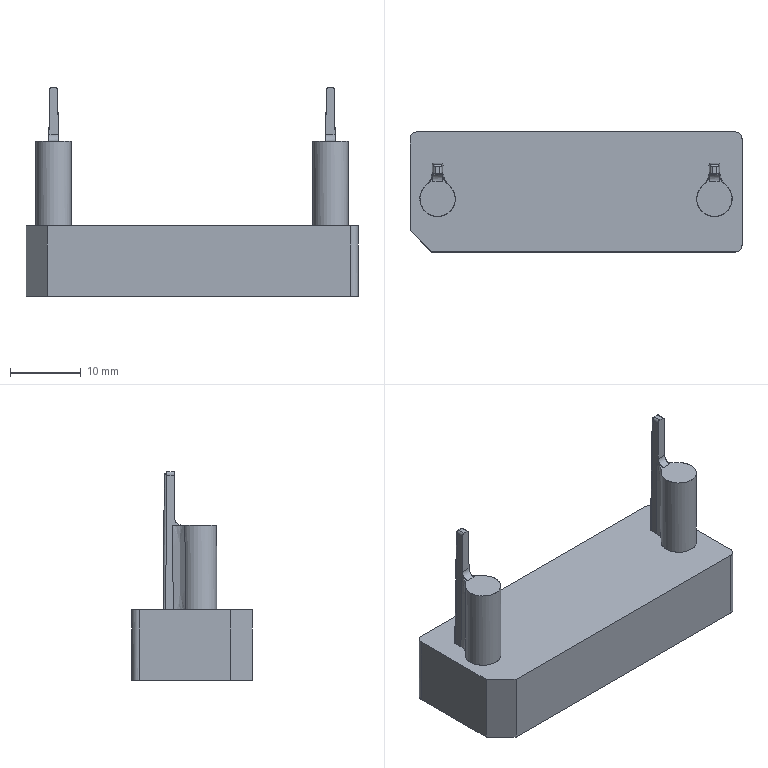NC program | PowerMill | posted with a generic post | part box 47 x 17 x 29.578 mm
Lines 11328 to 12336 of 293638:
N11425 M6
N11426 S18000 M03
N11427 G00 G90 X0.0 Y0.0
N11428 G43 Z10.798 H14
N11429
N11430 G05 P10000 R8
N11431 X21.1256 Y0.1265
N11432 Z0.908
N11433 G01 Z-0.292 F1200.0
N11434 X21.1142 Y0.1757 F2000.0
N11435 X21.0989 Y0.2239
N11436 X21.0799 Y0.2707
N11437 X21.0572 Y0.3158
N11438 X21.031 Y0.3591
N11439 X21.0015 Y0.4001
N11440 X20.9688 Y0.4387
N11441 X20.9333 Y0.4746
N11442 X20.895 Y0.5075
N11443 X20.8542 Y0.5374
N11444 X20.8112 Y0.5639
N11445 X20.7662 Y0.5869
N11446 X20.7196 Y0.6064
N11447 X20.6716 Y0.622
N11448 X20.6224 Y0.6339
N11449 X20.5725 Y0.6418
N11450 X20.5221 Y0.6458
N11451 X20.4716
N11452 X20.4212 Y0.6418
N11453 X20.3768 Y0.6349
N11454 X20.2929 Y0.6188
N11455 X20.2213 Y0.6083
N11456 X20.1571 Y0.6022
N11457 X20.094 Y0.599
N11458 X19.9708 Y0.5959
N11459 X19.8095 Y0.595
N11460 X19.4967 Y0.5949
N11461 X19.2215 Y0.5945
N11462 X19.1327 Y0.5963
N11463 X19.0442 Y0.602
N11464 X18.9562 Y0.6118
N11465 X18.8689 Y0.6254
N11466 X18.7825 Y0.643
N11467 X18.6971 Y0.6644
N11468 X18.6131 Y0.6896
N11469 X18.5304 Y0.7186
N11470 X18.4493 Y0.7512
N11471 X18.3699 Y0.7874
N11472 X18.2923 Y0.8272
N11473 X18.2163 Y0.8706
N11474 X18.1424 Y0.9174
N11475 X18.0707 Y0.9675
N11476 X18.0013 Y1.0209
N11477 X17.9345 Y1.0773
N11478 X17.8702 Y1.1367
N11479 X17.8087 Y1.1991
N11480 X17.75 Y1.2642
N11481 X17.6944 Y1.332
N11482 X17.6418 Y1.4022
N11483 X17.5925 Y1.4748
N11484 X17.5465 Y1.5496
N11485 X17.5041 Y1.6263
N11486 X17.4651 Y1.7049
N11487 X17.4298 Y1.7851
N11488 X17.3982 Y1.8667
N11489 X17.3704 Y1.9497
N11490 X17.3464 Y2.0338
N11491 X17.3262 Y2.119
N11492 X17.3098 Y2.2049
N11493 X17.2986 Y2.2821
N11494 X17.2908 Y2.3622
N11495 X17.2858 Y2.4512
N11496 X17.2838 Y2.5544
N11497 X17.2839 Y2.6866
N11498 X17.2846 Y3.3577
N11499 X17.2842 Y3.5211
N11500 X17.2858 Y3.6205
N11501 X17.2909 Y3.7136
N11502 X17.2994 Y3.8014
N11503 X17.3111 Y3.8849
N11504 X17.3262 Y3.9645
N11505 X17.3447 Y4.0428
N11506 X17.3689 Y4.1287
N11507 X17.3967 Y4.2126
N11508 X17.4279 Y4.2945
N11509 X17.4626 Y4.3742
N11510 X17.5006 Y4.4518
N11511 X17.5429 Y4.5289
N11512 X17.5885 Y4.604
N11513 X17.6376 Y4.6769
N11514 X17.6899 Y4.7476
N11515 X17.7454 Y4.8158
N11516 X17.8039 Y4.8815
N11517 X17.8654 Y4.9444
N11518 X17.9297 Y5.0045
N11519 X17.9951 Y5.0604
N11520 X18.063 Y5.1131
N11521 X18.1336 Y5.1629
N11522 X18.207 Y5.2099
N11523 X18.2831 Y5.2539
N11524 X18.3617 Y5.2947
N11525 X18.4429 Y5.3324
N11526 X18.5263 Y5.3668
N11527 X18.612 Y5.3977
N11528 X18.6997 Y5.4252
N11529 X18.7893 Y5.4491
N11530 X18.8806 Y5.4694
N11531 X18.9653 Y5.4846
N11532 X19.0519 Y5.4965
N11533 X19.1389 Y5.5046
N11534 X19.2326 Y5.5095
N11535 X19.325 Y5.5111
N11536 X19.4179 Y5.511
N11537 X19.9141 Y5.5102
N11538 X20.0031 Y5.508
N11539 X20.0929 Y5.5017
N11540 X20.1833 Y5.4914
N11541 X20.2739 Y5.4771
N11542 X20.3646 Y5.4587
N11543 X20.4551 Y5.4363
N11544 X20.5451 Y5.4099
N11545 X20.6343 Y5.3797
N11546 X20.7165 Y5.3478
N11547 X20.7971 Y5.3124
N11548 X20.8759 Y5.2733
N11549 X20.953 Y5.2307
N11550 X21.028 Y5.1847
N11551 X21.1008 Y5.1353
N11552 X21.1712 Y5.0827
N11553 X21.2392 Y5.027
N11554 X21.3045 Y4.9682
N11555 X21.3672 Y4.9066
N11556 X21.4262 Y4.843
N11557 X21.4823 Y4.7767
N11558 X21.5355 Y4.7077
N11559 X21.5856 Y4.6362
N11560 X21.6326 Y4.5622
N11561 X21.6761 Y4.4862
N11562 X21.716 Y4.4086
N11563 X21.7524 Y4.3293
N11564 X21.7851 Y4.2485
N11565 X21.8141 Y4.1661
N11566 X21.8395 Y4.0822
N11567 X21.8611 Y3.997
N11568 X21.8789 Y3.9106
N11569 X21.8929 Y3.8229
N11570 X21.903 Y3.7342
N11571 X21.9092 Y3.6445
N11572 X21.9114 Y3.5539
N11573 X21.9107 Y3.4626
N11574 X21.9103 Y3.2264
N11575 X21.9107 Y2.87
N11576 X21.9117 Y2.5975
N11577 X21.9107 Y2.492
N11578 X21.9063 Y2.3957
N11579 X21.8987 Y2.3063
N11580 X21.8878 Y2.2225
N11581 X21.8738 Y2.1433
N11582 X21.8564 Y2.065
N11583 X21.8334 Y1.9793
N11584 X21.8067 Y1.8952
N11585 X21.7764 Y1.8129
N11586 X21.7427 Y1.7326
N11587 X21.7054 Y1.6543
N11588 X21.6649 Y1.5782
N11589 X21.621 Y1.5041
N11590 X21.5723 Y1.4298
N11591 X21.5208 Y1.3582
N11592 X21.4664 Y1.2895
N11593 X21.4092 Y1.2236
N11594 X21.3493 Y1.1607
N11595 X21.2866 Y1.1006
N11596 X21.2204 Y1.0428
N11597 X21.1517 Y0.988
N11598 X21.0806 Y0.9365
N11599 X21.0073 Y0.8882
N11600 X20.9319 Y0.8433
N11601 X20.8546 Y0.802
N11602 X20.7754 Y0.7642
N11603 X20.6948 Y0.7301
N11604 X20.6126 Y0.6997
N11605 X20.529 Y0.6731
N11606 X20.4441 Y0.6502
N11607 X20.3768 Y0.6349
N11608 X20.328 Y0.6218
N11609 X20.2804 Y0.6049
N11610 X20.2343 Y0.5842
N11611 X20.1899 Y0.56
N11612 X20.1476 Y0.5324
N11613 X20.1076 Y0.5015
N11614 X20.0701 Y0.4676
N11615 X20.0355 Y0.4308
N11616 X20.0038 Y0.3914
N11617 X19.9754 Y0.3496
N11618 X19.9504 Y0.3057
N11619 X19.9289 Y0.26
N11620 X19.9111 Y0.2128
N11621 X19.897 Y0.1642
N11622 X19.8868 Y0.1147
N11623 X19.8806 Y0.0645
N11624 X19.8784 Y0.0141
N11625 X19.8801 Y-0.0364
N11626 X19.8858 Y-0.0866
N11627 X19.8942 Y-0.1308
N11628 X21.1239 Y0.1156 Z-0.312
N11629 X21.1128 Y0.1648
N11630 X21.0978 Y0.2131
N11631 X21.079 Y0.26
N11632 X21.0566 Y0.3053
N11633 X21.0306 Y0.3487
N11634 X21.0014 Y0.3899
N11635 X20.9689 Y0.4287
N11636 X20.9336 Y0.4647
N11637 X20.8955 Y0.4979
N11638 X20.8548 Y0.528
N11639 X20.812 Y0.5547
N11640 X20.7672 Y0.578
N11641 X20.7207 Y0.5977
N11642 X20.6727 Y0.6137
N11643 X20.6236 Y0.6258
N11644 X20.5737 Y0.634
N11645 X20.5234 Y0.6383
N11646 X20.4729 Y0.6386
N11647 X20.4225 Y0.6349
N11648 X20.378 Y0.6282
N11649 X20.3278 Y0.6189
N11650 X20.2419 Y0.607
N11651 X20.156 Y0.5992
N11652 X20.07 Y0.5953
N11653 X19.984 Y0.5948
N11654 X19.2215 Y0.5947
N11655 X19.1172 Y0.5963
N11656 X19.0237 Y0.6011
N11657 X18.9378 Y0.6091
N11658 X18.8579 Y0.6201
N11659 X18.7826 Y0.6342
N11660 X18.708 Y0.6516
N11661 X18.6213 Y0.6756
N11662 X18.5367 Y0.703
N11663 X18.4543 Y0.7339
N11664 X18.3743 Y0.7681
N11665 X18.2968 Y0.8055
N11666 X18.2218 Y0.846
N11667 X18.1489 Y0.8899
N11668 X18.0745 Y0.9391
N11669 X18.003 Y0.9913
N11670 X17.9344 Y1.0462
N11671 X17.8689 Y1.1037
N11672 X17.8067 Y1.1636
N11673 X17.7475 Y1.2259
N11674 X17.6898 Y1.2927
N11675 X17.6352 Y1.3619
N11676 X17.5839 Y1.4333
N11677 X17.536 Y1.5068
N11678 X17.4916 Y1.5823
N11679 X17.4508 Y1.6595
N11680 X17.4137 Y1.7383
N11681 X17.3802 Y1.8187
N11682 X17.3501 Y1.901
N11683 X17.3244 Y1.9824
N11684 X17.303 Y2.0632
N11685 X17.2872 Y2.1358
N11686 X17.2745 Y2.2051
N11687 X17.2638 Y2.2746
N11688 X17.2558 Y2.3446
N11689 X17.2509 Y2.4148
N11690 X17.2486 Y2.4853
N11691 X17.248 Y2.5558
N11692 Y2.6263
N11693 X17.2476 Y3.1941
N11694 X17.2472 Y3.521
N11695 X17.2485 Y3.6202
N11696 X17.2529 Y3.708
N11697 X17.2606 Y3.7893
N11698 X17.2727 Y3.8762
N11699 X17.2889 Y3.9625
N11700 X17.3089 Y4.048
N11701 X17.3328 Y4.1325
N11702 X17.3606 Y4.2158
N11703 X17.392 Y4.2976
N11704 X17.4272 Y4.3779
N11705 X17.4659 Y4.4565
N11706 X17.5082 Y4.5333
N11707 X17.554 Y4.608
N11708 X17.6031 Y4.6806
N11709 X17.6555 Y4.7509
N11710 X17.711 Y4.8187
N11711 X17.7695 Y4.8839
N11712 X17.8313 Y4.9469
N11713 X17.8956 Y5.0066
N11714 X17.9621 Y5.0631
N11715 X18.0308 Y5.1162
N11716 X18.1016 Y5.1661
N11717 X18.1788 Y5.2156
N11718 X18.2581 Y5.2617
N11719 X18.3395 Y5.3044
N11720 X18.4228 Y5.3437
N11721 X18.5078 Y5.3793
N11722 X18.5885 Y5.4092
N11723 X18.6702 Y5.4362
N11724 X18.7529 Y5.4598
N11725 X18.8367 Y5.4801
N11726 X18.923 Y5.4972
N11727 X19.0121 Y5.5108
N11728 X19.1042 Y5.521
N11729 X19.1995 Y5.5276
N11730 X19.2977 Y5.5306
N11731 X19.3976 Y5.5308
N11732 X19.9141 Y5.5307
N11733 X19.9966 Y5.5288
N11734 X20.0826 Y5.5228
N11735 X20.1727 Y5.5127
N11736 X20.2605 Y5.4993
N11737 X20.3508 Y5.4819
N11738 X20.4404 Y5.4606
N11739 X20.5289 Y5.4354
N11740 X20.616 Y5.4064
N11741 X20.7017 Y5.3738
N11742 X20.7857 Y5.3377
N11743 X20.8696 Y5.2975
N11744 X20.9502 Y5.2547
N11745 X21.0277 Y5.2091
N11746 X21.1021 Y5.1607
N11747 X21.1736 Y5.1096
N11748 X21.2423 Y5.0556
N11749 X21.3083 Y4.9988
N11750 X21.3716 Y4.9392
N11751 X21.4326 Y4.8765
N11752 X21.4908 Y4.8109
N11753 X21.546 Y4.7427
N11754 X21.598 Y4.672
N11755 X21.6467 Y4.5991
N11756 X21.6921 Y4.524
N11757 X21.734 Y4.4469
N11758 X21.7724 Y4.3679
N11759 X21.8072 Y4.2873
N11760 X21.8382 Y4.2053
N11761 X21.8655 Y4.1219
N11762 X21.8881 Y4.0405
N11763 X21.9071 Y3.9572
N11764 X21.9226 Y3.8715
N11765 X21.9345 Y3.7833
N11766 X21.9428 Y3.6928
N11767 X21.9473 Y3.5998
N11768 X21.9481 Y3.5043
N11769 X21.9472 Y3.1096
N11770 X21.9471 Y2.7232
N11771 X21.9475 Y2.5975
N11772 X21.9467 Y2.4897
N11773 X21.9428 Y2.3964
N11774 X21.9359 Y2.3124
N11775 X21.9258 Y2.2339
N11776 X21.9107 Y2.1474
N11777 X21.8915 Y2.0613
N11778 X21.8685 Y1.9758
N11779 X21.8421 Y1.8929
N11780 X21.812 Y1.8113
N11781 X21.7782 Y1.7311
N11782 X21.7407 Y1.6523
N11783 X21.6995 Y1.5752
N11784 X21.6547 Y1.4999
N11785 X21.6065 Y1.4265
N11786 X21.5549 Y1.3553
N11787 X21.5003 Y1.2867
N11788 X21.4426 Y1.2207
N11789 X21.3819 Y1.1573
N11790 X21.3184 Y1.0967
N11791 X21.2522 Y1.0391
N11792 X21.1835 Y0.9846
N11793 X21.1123 Y0.9332
N11794 X21.0389 Y0.8852
N11795 X20.9635 Y0.8406
N11796 X20.8861 Y0.7996
N11797 X20.8069 Y0.762
N11798 X20.726 Y0.7281
N11799 X20.6435 Y0.6978
N11800 X20.5597 Y0.6713
N11801 X20.4746 Y0.6486
N11802 X20.4137 Y0.6348
N11803 X20.378 Y0.6282
N11804 X20.3288 Y0.6171
N11805 X20.2805 Y0.6021
N11806 X20.2336 Y0.5833
N11807 X20.1883 Y0.5609
N11808 X20.1449 Y0.5349
N11809 X20.1037 Y0.5057
N11810 X20.0649 Y0.4732
N11811 X20.0289 Y0.4379
N11812 X19.9957 Y0.3998
N11813 X19.9656 Y0.3591
N11814 X19.9389 Y0.3163
N11815 X19.9156 Y0.2715
N11816 X19.8959 Y0.225
N11817 X19.8799 Y0.177
N11818 X19.8678 Y0.1279
N11819 X19.8596 Y0.078
N11820 X19.8553 Y0.0277
N11821 X19.855 Y-0.0228
N11822 X19.8587 Y-0.0732
N11823 X19.8654 Y-0.1177
N11824 X21.1241 Y0.1097 Z-0.332
N11825 X21.113 Y0.159
N11826 X21.0981 Y0.2073
N11827 X21.0794 Y0.2542
N11828 X21.057 Y0.2996
N11829 X21.0311 Y0.343
N11830 X21.0019 Y0.3843
N11831 X20.9696 Y0.4231
N11832 X20.9342 Y0.4592
N11833 X20.8962 Y0.4924
N11834 X20.8556 Y0.5225
N11835 X20.8128 Y0.5493
N11836 X20.768 Y0.5727
N11837 X20.7215 Y0.5925
N11838 X20.6736 Y0.6085
N11839 X20.6245 Y0.6207
N11840 X20.5746 Y0.629
N11841 X20.5243 Y0.6333
N11842 X20.4738 Y0.6337
N11843 X20.4234 Y0.63
N11844 X20.3789 Y0.6234
N11845 X20.3587 Y0.6197
N11846 X20.2731 Y0.608
N11847 X20.1846 Y0.5998
N11848 X20.0932 Y0.5954
N11849 X19.9986 Y0.5945
N11850 X19.6833 Y0.5944
N11851 X19.4371 Y0.5953
N11852 X19.2513 Y0.5949
N11853 X19.1478 Y0.5944
N11854 X19.0518 Y0.5973
N11855 X18.9618 Y0.6036
N11856 X18.8767 Y0.6133
N11857 X18.796 Y0.6263
N11858 X18.7172 Y0.6428
N11859 X18.6309 Y0.6648
N11860 X18.5461 Y0.6905
N11861 X18.463 Y0.7198
N11862 X18.3817 Y0.7527
N11863 X18.3024 Y0.7891
N11864 X18.2251 Y0.8289
N11865 X18.1498 Y0.8722
N11866 X18.0758 Y0.9193
N11867 X18.0041 Y0.9697
N11868 X17.9347 Y1.0233
N11869 X17.8678 Y1.08
N11870 X17.8036 Y1.1397
N11871 X17.7421 Y1.2023
N11872 X17.6836 Y1.2677
N11873 X17.628 Y1.3356
N11874 X17.5757 Y1.4059
N11875 X17.5266 Y1.4786
N11876 X17.4809 Y1.5534
N11877 X17.4386 Y1.6302
N11878 X17.3999 Y1.7088
N11879 X17.3657 Y1.787
N11880 X17.335 Y1.8668
N11881 X17.3074 Y1.9496
N11882 X17.2829 Y2.0354
N11883 X17.2617 Y2.1243
N11884 X17.2471 Y2.2004
N11885 X17.2357 Y2.2802
N11886 X17.2275 Y2.3655
N11887 X17.2224 Y2.4575
N11888 X17.2207 Y2.5587
N11889 X17.2214 Y2.6734
N11890 X17.2211 Y2.9073
N11891 X17.2206 Y3.1868
N11892 X17.2199 Y3.521
N11893 X17.2213 Y3.6149
N11894 X17.2266 Y3.707
N11895 X17.2356 Y3.7973
N11896 X17.2484 Y3.8859
N11897 X17.265 Y3.9727
N11898 X17.2852 Y4.058
N11899 X17.3091 Y4.1416
N11900 X17.3366 Y4.2236
N11901 X17.3678 Y4.3041
N11902 X17.4028 Y4.3832
N11903 X17.4415 Y4.4613
N11904 X17.4841 Y4.5381
N11905 X17.5301 Y4.6129
N11906 X17.5795 Y4.6855
N11907 X17.6321 Y4.7558
N11908 X17.6879 Y4.8237
N11909 X17.7467 Y4.889
N11910 X17.8084 Y4.9515
N11911 X17.8729 Y5.0111
N11912 X17.94 Y5.0677
N11913 X18.0095 Y5.1214
N11914 X18.0868 Y5.1764
N11915 X18.1652 Y5.2274
N11916 X18.2446 Y5.2743
N11917 X18.3248 Y5.3172
N11918 X18.4059 Y5.3561
N11919 X18.4862 Y5.3905
N11920 X18.5671 Y5.4217
N11921 X18.6491 Y5.4498
N11922 X18.7326 Y5.4746
N11923 X18.8179 Y5.4961
N11924 X18.9052 Y5.5142
N11925 X18.9948 Y5.5287
N11926 X19.0868 Y5.5396
N11927 X19.1815 Y5.5469
N11928 X19.2788 Y5.5506
N11929 X19.3785 Y5.5511
N11930 X19.9141 Y5.5506
N11931 X20.0006 Y5.5485
N11932 X20.0881 Y5.5425
N11933 X20.1774 Y5.5325
N11934 X20.2679 Y5.5184
N11935 X20.359 Y5.5002
N11936 X20.4499 Y5.478
N11937 X20.5397 Y5.4519
N11938 X20.6277 Y5.4223
N11939 X20.7131 Y5.3894
N11940 X20.7956 Y5.3534
N11941 X20.8755 Y5.3144
N11942 X20.9588 Y5.2694
N11943 X21.0397 Y5.2211
N11944 X21.1181 Y5.1697
N11945 X21.1938 Y5.1153
N11946 X21.2667 Y5.0581
N11947 X21.3328 Y5.0015
N11948 X21.3963 Y4.9419
N11949 X21.4573 Y4.8793
N11950 X21.5155 Y4.8138
N11951 X21.5708 Y4.7456
N11952 X21.623 Y4.6748
N11953 X21.672 Y4.6016
N11954 X21.7176 Y4.5263
N11955 X21.7598 Y4.449
N11956 X21.7983 Y4.3701
N11957 X21.8331 Y4.2896
N11958 X21.8642 Y4.2078
N11959 X21.891 Y4.1264
N11960 X21.914 Y4.0441
N11961 X21.9334 Y3.9603
N11962 X21.9492 Y3.875
N11963 X21.9612 Y3.788
N11964 X21.9694 Y3.6991
N11965 X21.9739 Y3.6081
N11966 X21.9747 Y3.5211
N11967 X21.9741 Y3.2959
N11968 X21.9746 Y3.0593
N11969 X21.9737 Y2.7677
N11970 X21.9741 Y2.5975
N11971 X21.9736 Y2.5078
N11972 X21.9703 Y2.4174
N11973 X21.9634 Y2.3272
N11974 X21.9531 Y2.2405
N11975 X21.9395 Y2.1574
N11976 X21.9227 Y2.0779
N11977 X21.9029 Y2.001
N11978 X21.88 Y1.925
N11979 X21.854 Y1.85
N11980 X21.8218 Y1.7689
N11981 X21.786 Y1.6893
N11982 X21.7465 Y1.6113
N11983 X21.7034 Y1.5351
N11984 X21.6568 Y1.4608
N11985 X21.6069 Y1.3886
N11986 X21.5536 Y1.3188
N11987 X21.4972 Y1.2513
N11988 X21.4378 Y1.1865
N11989 X21.3758 Y1.1248
N11990 X21.3111 Y1.0659
N11991 X21.2436 Y1.01
N11992 X21.1737 Y0.9572
N11993 X21.1014 Y0.9076
N11994 X21.0269 Y0.8613
N11995 X20.9503 Y0.8185
N11996 X20.8719 Y0.7792
N11997 X20.7918 Y0.7435
N11998 X20.7101 Y0.7116
N11999 X20.6271 Y0.6833
N12000 X20.5429 Y0.6589
N12001 X20.4577 Y0.6384
N12002 X20.4416 Y0.635
N12003 X20.3789 Y0.6234
N12004 X20.3296 Y0.6123
N12005 X20.2814 Y0.5974
N12006 X20.2344 Y0.5787
N12007 X20.1891 Y0.5563
N12008 X20.1457 Y0.5304
N12009 X20.1044 Y0.5012
N12010 X20.0656 Y0.4689
N12011 X20.0295 Y0.4335
N12012 X19.9963 Y0.3955
N12013 X19.9662 Y0.3549
N12014 X19.9393 Y0.3121
N12015 X19.916 Y0.2673
N12016 X19.8962 Y0.2208
N12017 X19.8802 Y0.1729
N12018 X19.868 Y0.1238
N12019 X19.8597 Y0.0739
N12020 X19.8554 Y0.0236
N12021 X19.855 Y-0.0269
N12022 X19.8587 Y-0.0773
N12023 X19.8652 Y-0.1218
N12024 X21.1254 Y0.1076 Z-0.352
N12025 X21.1142 Y0.1569
N12026 X21.0992 Y0.2052
N12027 X21.0804 Y0.2521
N12028 X21.058 Y0.2974
N12029 X21.0321 Y0.3408
N12030 X21.0028 Y0.382
N12031 X20.9704 Y0.4207
N12032 X20.935 Y0.4568
N12033 X20.8969 Y0.49
N12034 X20.8563 Y0.52
N12035 X20.8135 Y0.5468
N12036 X20.7686 Y0.5701
N12037 X20.7221 Y0.5898
N12038 X20.6742 Y0.6058
N12039 X20.6251 Y0.6179
N12040 X20.5752 Y0.6261
N12041 X20.5249 Y0.6304
N12042 X20.4743 Y0.6307
N12043 X20.424 Y0.627
N12044 X20.3795 Y0.6203
N12045 X20.3695 Y0.6185
N12046 X20.3048 Y0.6084
N12047 X20.2492 Y0.6028
N12048 X20.155 Y0.5975
N12049 X20.0438 Y0.5948
N12050 X19.9141 Y0.5943
N12051 X19.3369 Y0.5942
N12052 X19.1777
N12053 X19.0658 Y0.5963
N12054 X18.9723 Y0.601
N12055 X18.8894 Y0.6085
N12056 X18.8138 Y0.6188
N12057 X18.7422 Y0.6323
N12058 X18.6522 Y0.6532
N12059 X18.5652 Y0.6775
N12060 X18.4812 Y0.7049
N12061 X18.4 Y0.7355
N12062 X18.3218 Y0.7692
N12063 X18.2455 Y0.8062
N12064 X18.1686 Y0.8479
N12065 X18.0936 Y0.8931
N12066 X18.0208 Y0.9415
N12067 X17.9503 Y0.9933
N12068 X17.8821 Y1.0482
N12069 X17.8165 Y1.1062
N12070 X17.7535 Y1.1672
N12071 X17.6934 Y1.231
N12072 X17.6362 Y1.2975
N12073 X17.582 Y1.3666
N12074 X17.5311 Y1.438
N12075 X17.4835 Y1.5117
N12076 X17.4393 Y1.5874
N12077 X17.3987 Y1.665
N12078 X17.3616 Y1.7443
N12079 X17.3282 Y1.8252
N12080 X17.2985 Y1.9075
N12081 X17.2726 Y1.991
N12082 X17.2505 Y2.0757
N12083 X17.2345 Y2.1494
N12084 X17.2214 Y2.2236
N12085 X17.2114 Y2.2983
N12086 X17.2043 Y2.3761
N12087 X17.2001 Y2.4586
N12088 X17.1985 Y2.5341
N12089 X17.1983 Y2.6096
N12090 X17.1991 Y3.101
N12091 X17.1981 Y3.5211
N12092 X17.1996 Y3.6175
N12093 X17.2047 Y3.7105
N12094 X17.2135 Y3.8003
N12095 X17.2259 Y3.8871
N12096 X17.2417 Y3.971
N12097 X17.2609 Y4.0522
N12098 X17.2837 Y4.1317
N12099 X17.3121 Y4.2166
N12100 X17.3439 Y4.2992
N12101 X17.3791 Y4.3796
N12102 X17.4175 Y4.4576
N12103 X17.4591 Y4.5331
N12104 X17.5039 Y4.6062
N12105 X17.5535 Y4.6797
N12106 X17.6063 Y4.7507
N12107 X17.6622 Y4.8192
N12108 X17.7213 Y4.8854
N12109 X17.7836 Y4.9491
N12110 X17.8491 Y5.0105
N12111 X17.921 Y5.0723
N12112 X17.9951 Y5.1309
N12113 X18.0715 Y5.186
N12114 X18.1499 Y5.2378
N12115 X18.2301 Y5.286
N12116 X18.3121 Y5.3306
N12117 X18.3956 Y5.3715
N12118 X18.4806 Y5.4087
N12119 X18.5668 Y5.4421
N12120 X18.6542 Y5.4717
N12121 X18.7402 Y5.4967
N12122 X18.8271 Y5.5182
N12123 X18.9156 Y5.536
N12124 X19.0063 Y5.5503
N12125 X19.0993 Y5.5609
N12126 X19.1948 Y5.5678
N12127 X19.2931 Y5.5711
N12128 X19.3938 Y5.5713
N12129 X19.9141 Y5.5707
N12130 X20.0009 Y5.5686
N12131 X20.0887 Y5.5625
N12132 X20.1782 Y5.5525
N12133 X20.2688 Y5.5383
N12134 X20.3599 Y5.5201
N12135 X20.4509 Y5.4978
N12136 X20.5408 Y5.4717
N12137 X20.6289 Y5.442
N12138 X20.7146 Y5.4089
N12139 X20.7974 Y5.3728
N12140 X20.8777 Y5.3335
N12141 X20.9601 Y5.2889
N12142 X21.0406 Y5.2406
N12143 X21.1192 Y5.1889
N12144 X21.1956 Y5.1339
N12145 X21.2699 Y5.0755
N12146 X21.3417 Y5.0139
N12147 X21.4087 Y4.9516
N12148 X21.4706 Y4.8888
N12149 X21.5276 Y4.8255
N12150 X21.5818 Y4.7597
N12151 X21.635 Y4.689
N12152 X21.6846 Y4.6165
N12153 X21.7307 Y4.5421
N12154 X21.7731 Y4.4662
N12155 X21.8117 Y4.3888
N12156 X21.8465 Y4.3101
N12157 X21.8776 Y4.2302
N12158 X21.903 Y4.1559
N12159 X21.9257 Y4.0807
N12160 X21.9455 Y4.0047
N12161 X21.962 Y3.928
N12162 X21.9751 Y3.8503
N12163 X21.9854 Y3.7674
N12164 X21.9923 Y3.6797
N12165 X21.9957 Y3.5939
N12166 X21.9964 Y3.5102
N12167 X21.9963 Y2.9438
N12168 X21.9962 Y2.8824
N12169 Y2.8209
N12170 X21.9961 Y2.7594
N12171 X21.9959 Y2.691
N12172 X21.9957 Y2.6295
N12173 X21.9953 Y2.5681
N12174 X21.9948 Y2.5066
N12175 X21.994 Y2.4452
N12176 X21.9925 Y2.3884
N12177 X21.9884 Y2.3317
N12178 X21.9817 Y2.2753
N12179 X21.973 Y2.2174
N12180 X21.96 Y2.1465
N12181 X21.9413 Y2.0617
N12182 X21.9241 Y1.9949
N12183 X21.9079 Y1.9404
N12184 X21.8898 Y1.8866
N12185 X21.8572 Y1.8012
N12186 X21.8215 Y1.7185
N12187 X21.7827 Y1.6386
N12188 X21.741 Y1.5616
N12189 X21.6964 Y1.4875
N12190 X21.6487 Y1.416
N12191 X21.5968 Y1.3453
N12192 X21.5416 Y1.2769
N12193 X21.4832 Y1.2109
N12194 X21.4218 Y1.1474
N12195 X21.3601 Y1.0892
N12196 X21.295 Y1.0333
N12197 X21.2264 Y0.9795
N12198 X21.1542 Y0.9281
N12199 X21.0784 Y0.8789
N12200 X21.0064 Y0.8365
N12201 X20.9316 Y0.797
N12202 X20.8537 Y0.7604
N12203 X20.7728 Y0.7267
N12204 X20.6889 Y0.6961
N12205 X20.6107 Y0.6711
N12206 X20.5377 Y0.6516
N12207 X20.4688 Y0.6369
N12208 X20.4645 Y0.6361
N12209 X20.3795 Y0.6203
N12210 X20.3302 Y0.6092
N12211 X20.282 Y0.5942
N12212 X20.2351 Y0.5754
N12213 X20.1898 Y0.553
N12214 X20.1464 Y0.527
N12215 X20.1052 Y0.4978
N12216 X20.0664 Y0.4653
N12217 X20.0303 Y0.43
N12218 X19.9971 Y0.3919
N12219 X19.9671 Y0.3513
N12220 X19.9403 Y0.3084
N12221 X19.917 Y0.2636
N12222 X19.8973 Y0.2171
N12223 X19.8814 Y0.1691
N12224 X19.8692 Y0.12
N12225 X19.861 Y0.0702
N12226 X19.8567 Y0.0198
N12227 X19.8564 Y-0.0307
N12228 X19.8602 Y-0.0811
N12229 X19.8668 Y-0.1255
N12230 X21.1068 Y0.0762 Z-0.372
N12231 X21.0975 Y0.1258
N12232 X21.0843 Y0.1746
N12233 X21.0672 Y0.2221
N12234 X21.0465 Y0.2682
N12235 X21.0221 Y0.3125
N12236 X20.9944 Y0.3548
N12237 X20.9634 Y0.3947
N12238 X20.9294 Y0.4321
N12239 X20.8925 Y0.4666
N12240 X20.853 Y0.4981
N12241 X20.8112 Y0.5264
N12242 X20.7672 Y0.5514
N12243 X20.7214 Y0.5727
N12244 X20.6741 Y0.5904
N12245 X20.6255 Y0.6044
N12246 X20.576 Y0.6144
N12247 X20.5258 Y0.6205
N12248 X20.4753 Y0.6226
N12249 X20.4249 Y0.6208
N12250 X20.3802 Y0.6158
N12251 X20.3287 Y0.6081
N12252 X20.2636 Y0.6019
N12253 X20.1986 Y0.5985
N12254 X20.0833 Y0.5953
N12255 X19.9321 Y0.5943
N12256 X19.5641 Y0.5942
N12257 X19.3369 Y0.5941
N12258 X19.2094 Y0.5933
N12259 X19.1193 Y0.5938
N12260 X19.0542 Y0.5957
N12261 X18.9891 Y0.5981
N12262 X18.9241 Y0.6023
N12263 X18.8593 Y0.6098
N12264 X18.7949 Y0.6197
N12265 X18.7307 Y0.6305
N12266 X18.6611 Y0.6453
N12267 X18.5847 Y0.6655
N12268 X18.5038 Y0.6906
N12269 X18.4194 Y0.7206
N12270 X18.3397 Y0.7529
N12271 X18.2628 Y0.7882
N12272 X18.1848 Y0.8284
N12273 X18.1088 Y0.8721
N12274 X18.0347 Y0.9193
N12275 X17.9629 Y0.9697
N12276 X17.8935 Y1.0234
N12277 X17.8266 Y1.0802
N12278 X17.7623 Y1.1399
N12279 X17.7008 Y1.2026
N12280 X17.6423 Y1.2679
N12281 X17.5868 Y1.3359
N12282 X17.5344 Y1.4063
N12283 X17.4855 Y1.4787
N12284 X17.4399 Y1.5534
N12285 X17.3978 Y1.63
N12286 X17.3592 Y1.7085
N12287 X17.3241 Y1.7889
N12288 X17.2927 Y1.8708
N12289 X17.265 Y1.9542
N12290 X17.2412 Y2.0388
N12291 X17.2212 Y2.1245
N12292 X17.205 Y2.2111
N12293 X17.1943 Y2.2868
N12294 X17.1869 Y2.3663
N12295 X17.1822 Y2.4557
N12296 X17.1803 Y2.562
N12297 X17.1802 Y2.7102
N12298 X17.1801 Y3.0593
N12299 X17.1809 Y3.3348
N12300 X17.1802 Y3.5211
N12301 X17.181 Y3.6149
N12302 X17.1857 Y3.7064
N12303 X17.1942 Y3.7957
N12304 X17.2063 Y3.8825
N12305 X17.222 Y3.9671
N12306 X17.2413 Y4.0494
N12307 X17.2641 Y4.1298
N12308 X17.2921 Y4.2138
N12309 X17.3238 Y4.2963
N12310 X17.3591 Y4.3771
N12311 X17.398 Y4.4559
N12312 X17.4402 Y4.5327
N12313 X17.4858 Y4.6073
N12314 X17.5346 Y4.6796
N12315 X17.5866 Y4.7494
N12316 X17.6417 Y4.8169
N12317 X17.7044 Y4.8877
N12318 X17.77 Y4.9556
N12319 X17.8382 Y5.0206
N12320 X17.909 Y5.0826
N12321 X17.9823 Y5.1413
N12322 X18.0578 Y5.1968
N12323 X18.1355 Y5.2488
N12324 X18.2151 Y5.2975
N12325 X18.2967 Y5.3426
N12326 X18.38 Y5.3842
N12327 X18.4652 Y5.4222
N12328 X18.5516 Y5.4565
N12329 X18.6391 Y5.4868
N12330 X18.7275 Y5.5133
N12331 X18.8118 Y5.5348
N12332 X18.8969 Y5.5529
N12333 X18.9832 Y5.5675
N12334 X19.073 Y5.5787
N12335 X19.166 Y5.5864
N12336 X19.2593 Y5.5904
N12337 X19.3521 Y5.5912
N12338 X19.9141 Y5.5902
N12339 X20.0051 Y5.5879
N12340 X20.0958 Y5.5817
N12341 X20.1863 Y5.5714
N12342 X20.2766 Y5.5572
N12343 X20.3664 Y5.539
N12344 X20.4557 Y5.5169
N12345 X20.5444 Y5.4908
N12346 X20.6323 Y5.4608
N12347 X20.7193 Y5.4268
N12348 X20.8053 Y5.389
N12349 X20.8863 Y5.3492
N12350 X20.9665 Y5.3054
N12351 X21.0458 Y5.2576
N12352 X21.1239 Y5.2059
N12353 X21.2004 Y5.1505
N12354 X21.2747 Y5.0917
N12355 X21.3465 Y5.0299
N12356 X21.4152 Y4.9655
N12357 X21.4805 Y4.8988
N12358 X21.5421 Y4.8302
N12359 X21.6 Y4.7601
N12360 X21.6527 Y4.6901
N12361 X21.7022 Y4.618
N12362 X21.7484 Y4.5437
N12363 X21.7911 Y4.4673
N12364 X21.8303 Y4.3891
N12365 X21.8659 Y4.3092
N12366 X21.8978 Y4.2276
N12367 X21.926 Y4.1447
N12368 X21.9503 Y4.0606
N12369 X21.9708 Y3.9755
N12370 X21.9874 Y3.8896
N12371 X21.9992 Y3.8104
N12372 X22.0075 Y3.7308
N12373 X22.0128 Y3.6465
N12374 X22.0149 Y3.5664
N12375 X22.0151 Y3.4863
N12376 X22.0148 Y2.5975
N12377 X22.0139 Y2.4825
N12378 X22.0105 Y2.3921
N12379 X22.0043 Y2.314
N12380 X21.9953 Y2.2429
N12381 X21.9797 Y2.1531
N12382 X21.9605 Y2.0656
N12383 X21.9378 Y1.9805
N12384 X21.9118 Y1.8978
N12385 X21.8825 Y1.8176
N12386 X21.8496 Y1.7391
N12387 X21.8119 Y1.6591
N12388 X21.771 Y1.5815
N12389 X21.7268 Y1.5063
N12390 X21.6795 Y1.4335
N12391 X21.6284 Y1.3622
N12392 X21.5741 Y1.2934
N12393 X21.5168 Y1.2272
N12394 X21.4565 Y1.1636
N12395 X21.3934 Y1.1028
N12396 X21.3276 Y1.0449
N12397 X21.2591 Y0.99
N12398 X21.1882 Y0.9383
N12399 X21.115 Y0.8899
N12400 X21.0397 Y0.8449
N12401 X20.9624 Y0.8033
N12402 X20.8834 Y0.7654
N12403 X20.8028 Y0.731
N12404 X20.7207 Y0.7004
N12405 X20.6373 Y0.6736
N12406 X20.5527 Y0.6505
N12407 X20.4841 Y0.6348
N12408 X20.4008 Y0.6188
N12409 X20.3802 Y0.6158
N12410 X20.3305 Y0.6064
N12411 X20.2818 Y0.5932
N12412 X20.2342 Y0.5761
N12413 X20.1881 Y0.5554
N12414 X20.1438 Y0.531
N12415 X20.1015 Y0.5033
N12416 X20.0616 Y0.4723
N12417 X20.0243 Y0.4383
N12418 X19.9897 Y0.4014
N12419 X19.9582 Y0.3619
N12420 X19.9299 Y0.3201
N12421 X19.905 Y0.2761
N12422 X19.8836 Y0.2304
N12423 X19.8659 Y0.183
N12424 X19.852 Y0.1344
N12425 X19.8419 Y0.0849
N12426 X19.8358 Y0.0347
N12427 X19.8337 Y-0.0158
N12428 X19.8356 Y-0.0662
N12429 X19.8406 Y-0.1109
N12430 X21.1055 Y0.0723 Z-0.392
N12431 X21.0963 Y0.122
N12432 X21.0832 Y0.1708
N12433 X21.0663 Y0.2184